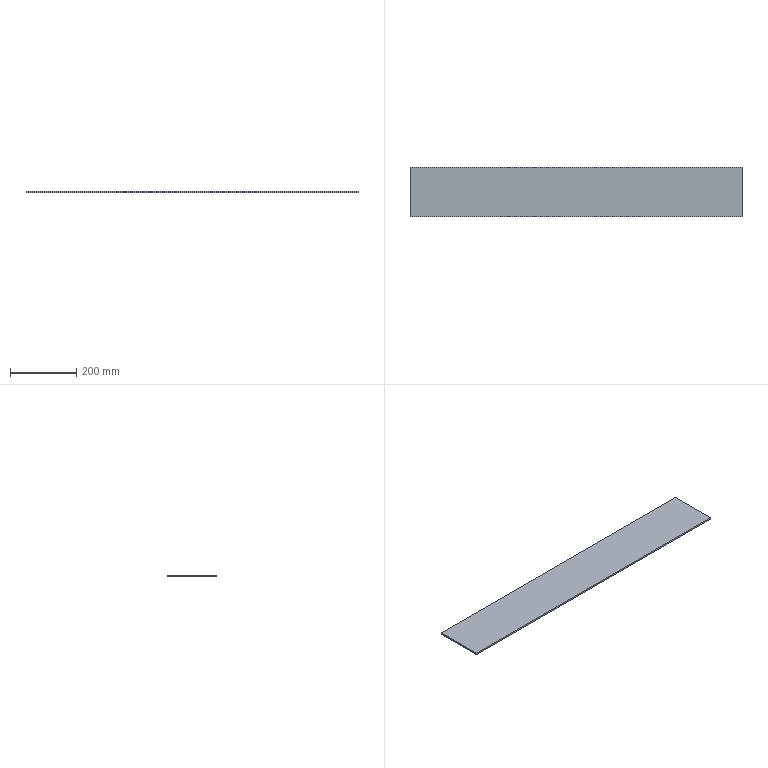Part | SolidWorks | features Extrusion 1 | 1 solid | 6 faces | box 1000 x 150 x 5 mm | volume 750000 mm3 | plane 6
STEP:
#1=CARTESIAN_POINT('',(0.,150.,0.));
#2=VERTEX_POINT('',#1);
#3=CARTESIAN_POINT('',(0.,0.,0.));
#4=VERTEX_POINT('',#3);
#5=CARTESIAN_POINT('',(0.,0.,0.));
#6=DIRECTION('',(0.,-1.,0.));
#7=VECTOR('',#6,1000.);
#8=LINE('',#5,#7);
#9=EDGE_CURVE('',#2,#4,#8,.T.);
#10=ORIENTED_EDGE('',*,*,#9,.T.);
#11=CARTESIAN_POINT('',(0.,0.,5.));
#12=VERTEX_POINT('',#11);
#13=CARTESIAN_POINT('',(0.,0.,5.));
#14=DIRECTION('',(0.,0.,-1.));
#15=VECTOR('',#14,1000.);
#16=LINE('',#13,#15);
#17=EDGE_CURVE('',#12,#4,#16,.T.);
#18=ORIENTED_EDGE('',*,*,#17,.F.);
#19=CARTESIAN_POINT('',(0.,150.,5.));
#20=VERTEX_POINT('',#19);
#21=CARTESIAN_POINT('',(0.,0.,5.));
#22=DIRECTION('',(0.,-1.,0.));
#23=VECTOR('',#22,1000.);
#24=LINE('',#21,#23);
#25=EDGE_CURVE('',#20,#12,#24,.T.);
#26=ORIENTED_EDGE('',*,*,#25,.F.);
#27=CARTESIAN_POINT('',(0.,150.,5.));
#28=DIRECTION('',(0.,0.,-1.));
#29=VECTOR('',#28,1000.);
#30=LINE('',#27,#29);
#31=EDGE_CURVE('',#20,#2,#30,.T.);
#32=ORIENTED_EDGE('',*,*,#31,.T.);
#33=EDGE_LOOP('',(#10,#18,#26,#32));
#34=FACE_OUTER_BOUND('',#33,.T.);
#35=CARTESIAN_POINT('',(0.,0.,5.));
#36=DIRECTION('',(1.,0.,0.));
#37=DIRECTION('',(0.,0.,-1.));
#38=AXIS2_PLACEMENT_3D('',#35,#36,#37);
#39=PLANE('',#38);
#40=ADVANCED_FACE('',(#34),#39,.F.);
#41=CARTESIAN_POINT('',(1000.,0.,0.));
#42=VERTEX_POINT('',#41);
#43=CARTESIAN_POINT('',(0.,0.,0.));
#44=DIRECTION('',(1.,0.,0.));
#45=VECTOR('',#44,1000.);
#46=LINE('',#43,#45);
#47=EDGE_CURVE('',#4,#42,#46,.T.);
#48=ORIENTED_EDGE('',*,*,#47,.T.);
#49=CARTESIAN_POINT('',(1000.,0.,5.));
#50=VERTEX_POINT('',#49);
#51=CARTESIAN_POINT('',(1000.,0.,5.));
#52=DIRECTION('',(0.,0.,-1.));
#53=VECTOR('',#52,1000.);
#54=LINE('',#51,#53);
#55=EDGE_CURVE('',#50,#42,#54,.T.);
#56=ORIENTED_EDGE('',*,*,#55,.F.);
#57=CARTESIAN_POINT('',(0.,0.,5.));
#58=DIRECTION('',(1.,0.,0.));
#59=VECTOR('',#58,1000.);
#60=LINE('',#57,#59);
#61=EDGE_CURVE('',#12,#50,#60,.T.);
#62=ORIENTED_EDGE('',*,*,#61,.F.);
#63=ORIENTED_EDGE('',*,*,#17,.T.);
#64=EDGE_LOOP('',(#48,#56,#62,#63));
#65=FACE_OUTER_BOUND('',#64,.T.);
#66=CARTESIAN_POINT('',(0.,0.,5.));
#67=DIRECTION('',(0.,1.,0.));
#68=DIRECTION('',(0.,0.,1.));
#69=AXIS2_PLACEMENT_3D('',#66,#67,#68);
#70=PLANE('',#69);
#71=ADVANCED_FACE('',(#65),#70,.F.);
#72=CARTESIAN_POINT('',(1000.,150.,0.));
#73=VERTEX_POINT('',#72);
#74=CARTESIAN_POINT('',(1000.,0.,0.));
#75=DIRECTION('',(0.,1.,0.));
#76=VECTOR('',#75,1000.);
#77=LINE('',#74,#76);
#78=EDGE_CURVE('',#42,#73,#77,.T.);
#79=ORIENTED_EDGE('',*,*,#78,.T.);
#80=CARTESIAN_POINT('',(1000.,150.,5.));
#81=VERTEX_POINT('',#80);
#82=CARTESIAN_POINT('',(1000.,150.,5.));
#83=DIRECTION('',(0.,0.,-1.));
#84=VECTOR('',#83,1000.);
#85=LINE('',#82,#84);
#86=EDGE_CURVE('',#81,#73,#85,.T.);
#87=ORIENTED_EDGE('',*,*,#86,.F.);
#88=CARTESIAN_POINT('',(1000.,0.,5.));
#89=DIRECTION('',(0.,1.,0.));
#90=VECTOR('',#89,1000.);
#91=LINE('',#88,#90);
#92=EDGE_CURVE('',#50,#81,#91,.T.);
#93=ORIENTED_EDGE('',*,*,#92,.F.);
#94=ORIENTED_EDGE('',*,*,#55,.T.);
#95=EDGE_LOOP('',(#79,#87,#93,#94));
#96=FACE_OUTER_BOUND('',#95,.T.);
#97=CARTESIAN_POINT('',(1000.,0.,5.));
#98=DIRECTION('',(-1.,0.,0.));
#99=DIRECTION('',(0.,0.,1.));
#100=AXIS2_PLACEMENT_3D('',#97,#98,#99);
#101=PLANE('',#100);
#102=ADVANCED_FACE('',(#96),#101,.F.);
#103=CARTESIAN_POINT('',(0.,150.,0.));
#104=DIRECTION('',(-1.,0.,0.));
#105=VECTOR('',#104,1000.);
#106=LINE('',#103,#105);
#107=EDGE_CURVE('',#73,#2,#106,.T.);
#108=ORIENTED_EDGE('',*,*,#107,.T.);
#109=ORIENTED_EDGE('',*,*,#31,.F.);
#110=CARTESIAN_POINT('',(0.,150.,5.));
#111=DIRECTION('',(-1.,0.,0.));
#112=VECTOR('',#111,1000.);
#113=LINE('',#110,#112);
#114=EDGE_CURVE('',#81,#20,#113,.T.);
#115=ORIENTED_EDGE('',*,*,#114,.F.);
#116=ORIENTED_EDGE('',*,*,#86,.T.);
#117=EDGE_LOOP('',(#108,#109,#115,#116));
#118=FACE_OUTER_BOUND('',#117,.T.);
#119=CARTESIAN_POINT('',(0.,150.,5.));
#120=DIRECTION('',(0.,-1.,0.));
#121=DIRECTION('',(0.,0.,-1.));
#122=AXIS2_PLACEMENT_3D('',#119,#120,#121);
#123=PLANE('',#122);
#124=ADVANCED_FACE('',(#118),#123,.F.);
#125=ORIENTED_EDGE('',*,*,#25,.T.);
#126=ORIENTED_EDGE('',*,*,#61,.T.);
#127=ORIENTED_EDGE('',*,*,#92,.T.);
#128=ORIENTED_EDGE('',*,*,#114,.T.);
#129=EDGE_LOOP('',(#125,#126,#127,#128));
#130=FACE_OUTER_BOUND('',#129,.T.);
#131=CARTESIAN_POINT('',(0.,0.,5.));
#132=DIRECTION('',(0.,0.,-1.));
#133=DIRECTION('',(-1.,0.,0.));
#134=AXIS2_PLACEMENT_3D('',#131,#132,#133);
#135=PLANE('',#134);
#136=ADVANCED_FACE('',(#130),#135,.F.);
#137=ORIENTED_EDGE('',*,*,#9,.F.);
#138=ORIENTED_EDGE('',*,*,#107,.F.);
#139=ORIENTED_EDGE('',*,*,#78,.F.);
#140=ORIENTED_EDGE('',*,*,#47,.F.);
#141=EDGE_LOOP('',(#137,#138,#139,#140));
#142=FACE_OUTER_BOUND('',#141,.T.);
#143=CARTESIAN_POINT('',(0.,0.,0.));
#144=DIRECTION('',(0.,0.,-1.));
#145=DIRECTION('',(-1.,0.,0.));
#146=AXIS2_PLACEMENT_3D('',#143,#144,#145);
#147=PLANE('',#146);
#148=ADVANCED_FACE('',(#142),#147,.T.);
#149=CLOSED_SHELL('',(#40,#71,#102,#124,#136,#148));
#150=MANIFOLD_SOLID_BREP('',#149);
#151=CARTESIAN_POINT('',(0.,0.,0.));
#152=DIRECTION('',(0.,0.,1.));
#153=DIRECTION('',(1.,0.,0.));
#154=AXIS2_PLACEMENT_3D('',#151,#152,#153);
#155=(LENGTH_UNIT()NAMED_UNIT(*)SI_UNIT(.MILLI.,.METRE.));
#156=UNCERTAINTY_MEASURE_WITH_UNIT(LENGTH_MEASURE(0.00001),#155,'','');
#157=(NAMED_UNIT(*)PLANE_ANGLE_UNIT()SI_UNIT($,.RADIAN.));
#158=(NAMED_UNIT(*)SI_UNIT($,.STERADIAN.)SOLID_ANGLE_UNIT());
#159=(GEOMETRIC_REPRESENTATION_CONTEXT(3)GLOBAL_UNCERTAINTY_ASSIGNED_CONTEXT((#156))GLOBAL_UNIT_ASSIGNED_CONTEXT((#155,#157,#158))REPRESENTATION_CONTEXT('',''));
#160=ADVANCED_BREP_SHAPE_REPRESENTATION('',(#150,#154),#159);